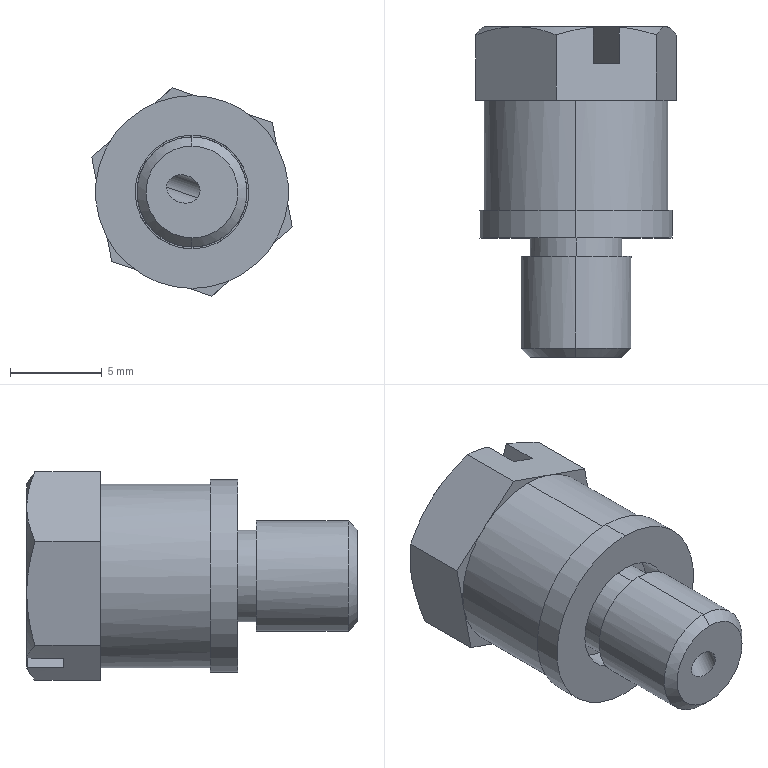Part | SolidWorks | features BaseBody 1 | 1 solid | 44 faces | box 10.905 x 18.006 x 11.342 mm | volume 1063 mm3 | plane 22 | cylinder 12 | cone 10 | commonest cylinder face diameters 1.5 x2 5 x2 6 x2 6.2 x2 10 x2 10.5 x2